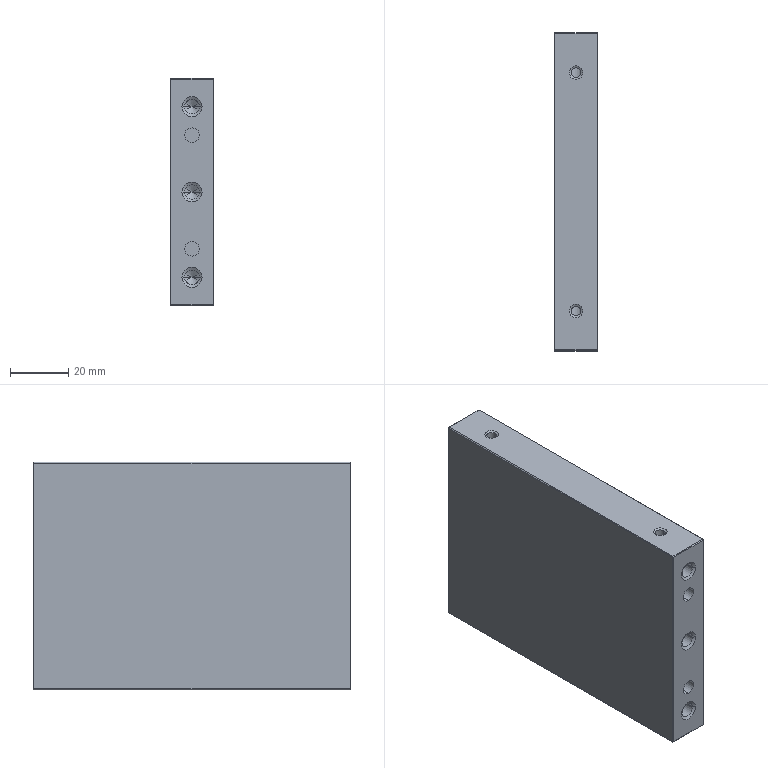Part | NX | 1 solid | 93 faces | box 15 x 109 x 78 mm | volume 124204 mm3 | cylinder 40 | cone 32 | plane 21 | commonest cylinder face diameters 5 x32 3.3 x8